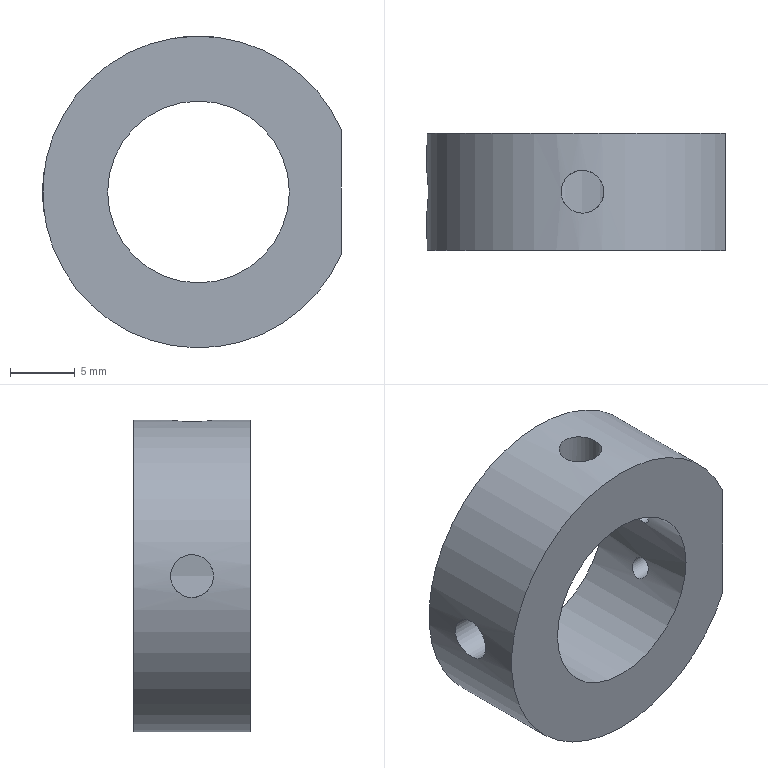Part | NX | 1 solid | 9 faces | box 23 x 9 x 24 mm | volume 2524 mm3 | cylinder 6 | plane 3 | commonest cylinder face diameters 1.6 x2 3.3 x2 14 x1 24 x1
STEP:
#1=CARTESIAN_POINT('',(11.,4.5,-4.796));
#2=VERTEX_POINT('',#1);
#3=CARTESIAN_POINT('',(11.,4.5,4.796));
#4=VERTEX_POINT('',#3);
#5=CARTESIAN_POINT('',(11.,4.5,10.));
#6=DIRECTION('',(0.,0.,1.));
#7=VECTOR('',#6,1000.);
#8=LINE('',#5,#7);
#9=EDGE_CURVE('',#2,#4,#8,.T.);
#10=ORIENTED_EDGE('',*,*,#9,.F.);
#11=CARTESIAN_POINT('',(0.,4.5,0.));
#12=DIRECTION('',(0.,1.,0.));
#13=DIRECTION('',(0.,0.,1.));
#14=AXIS2_PLACEMENT_3D('',#11,#12,#13);
#15=CIRCLE('',#14,12.);
#16=EDGE_CURVE('',#2,#4,#15,.T.);
#17=ORIENTED_EDGE('',*,*,#16,.T.);
#18=EDGE_LOOP('',(#10,#17));
#19=FACE_BOUND('',#18,.T.);
#20=CARTESIAN_POINT('',(0.,4.5,7.));
#21=VERTEX_POINT('',#20);
#22=CARTESIAN_POINT('',(0.,4.5,0.));
#23=DIRECTION('',(0.,1.,0.));
#24=DIRECTION('',(0.,0.,1.));
#25=AXIS2_PLACEMENT_3D('',#22,#23,#24);
#26=CIRCLE('',#25,7.);
#27=EDGE_CURVE('',#21,#21,#26,.T.);
#28=ORIENTED_EDGE('',*,*,#27,.F.);
#29=EDGE_LOOP('',(#28));
#30=FACE_BOUND('',#29,.T.);
#31=CARTESIAN_POINT('',(0.,4.5,0.));
#32=DIRECTION('',(0.,1.,0.));
#33=DIRECTION('',(0.,0.,1.));
#34=AXIS2_PLACEMENT_3D('',#31,#32,#33);
#35=PLANE('',#34);
#36=ADVANCED_FACE('',(#19,#30),#35,.T.);
#37=CARTESIAN_POINT('',(11.,-4.5,-4.796));
#38=VERTEX_POINT('',#37);
#39=CARTESIAN_POINT('',(11.,-4.5,4.796));
#40=VERTEX_POINT('',#39);
#41=CARTESIAN_POINT('',(0.,-4.5,0.));
#42=DIRECTION('',(0.,1.,0.));
#43=DIRECTION('',(0.,0.,1.));
#44=AXIS2_PLACEMENT_3D('',#41,#42,#43);
#45=CIRCLE('',#44,12.);
#46=EDGE_CURVE('',#38,#40,#45,.T.);
#47=ORIENTED_EDGE('',*,*,#46,.F.);
#48=CARTESIAN_POINT('',(11.,-4.5,0.));
#49=DIRECTION('',(0.,0.,1.));
#50=VECTOR('',#49,1000.);
#51=LINE('',#48,#50);
#52=EDGE_CURVE('',#38,#40,#51,.T.);
#53=ORIENTED_EDGE('',*,*,#52,.T.);
#54=EDGE_LOOP('',(#47,#53));
#55=FACE_BOUND('',#54,.T.);
#56=CARTESIAN_POINT('',(0.,-4.5,7.));
#57=VERTEX_POINT('',#56);
#58=CARTESIAN_POINT('',(0.,-4.5,0.));
#59=DIRECTION('',(0.,1.,0.));
#60=DIRECTION('',(0.,0.,1.));
#61=AXIS2_PLACEMENT_3D('',#58,#59,#60);
#62=CIRCLE('',#61,7.);
#63=EDGE_CURVE('',#57,#57,#62,.T.);
#64=ORIENTED_EDGE('',*,*,#63,.T.);
#65=EDGE_LOOP('',(#64));
#66=FACE_BOUND('',#65,.T.);
#67=CARTESIAN_POINT('',(0.,-4.5,0.));
#68=DIRECTION('',(0.,1.,0.));
#69=DIRECTION('',(0.,0.,1.));
#70=AXIS2_PLACEMENT_3D('',#67,#68,#69);
#71=PLANE('',#70);
#72=ADVANCED_FACE('',(#55,#66),#71,.F.);
#73=CARTESIAN_POINT('',(-12.,-1.65,0.));
#74=VERTEX_POINT('',#73);
#75=CARTESIAN_POINT('',(-11.943,-1.292,1.294));
#76=CARTESIAN_POINT('',(-12.028,-1.829,-0.000316));
#77=CARTESIAN_POINT('',(-11.943,-1.292,-1.293));
#78=CARTESIAN_POINT('',(-11.857,-0.001514,-1.828));
#79=CARTESIAN_POINT('',(-11.943,1.293,-1.294));
#80=CARTESIAN_POINT('',(-12.028,1.828,-0.0004038));
#81=CARTESIAN_POINT('',(-11.943,1.294,1.291));
#82=CARTESIAN_POINT('',(-11.857,0.00157,1.829));
#83=CARTESIAN_POINT('',(-11.943,-1.292,1.294));
#84=CARTESIAN_POINT('',(-12.028,-1.829,-0.000316));
#85=CARTESIAN_POINT('',(-11.943,-1.292,-1.293));
#86=B_SPLINE_CURVE_WITH_KNOTS('',3,(#75,#76,#77,#78,#79,#80,#81,#82,#83,#84,#85),.UNSPECIFIED.,.T.,.F.,(1,1,1,1,1,1,1,1,1,1,1,1,1,1,1),(-0.003873,-0.002582,-0.001291,0.,0.001291,0.002582,0.003873,0.005164,0.006455,0.007746,0.009037,0.01033,0.01162,0.01291,0.0142),.UNSPECIFIED.);
#87=EDGE_CURVE('',#74,#74,#86,.T.);
#88=ORIENTED_EDGE('',*,*,#87,.T.);
#89=EDGE_LOOP('',(#88));
#90=FACE_BOUND('',#89,.T.);
#91=CARTESIAN_POINT('',(0.,-1.65,12.));
#92=VERTEX_POINT('',#91);
#93=CARTESIAN_POINT('',(1.294,-1.292,11.943));
#94=CARTESIAN_POINT('',(-0.000316,-1.829,12.028));
#95=CARTESIAN_POINT('',(-1.293,-1.292,11.943));
#96=CARTESIAN_POINT('',(-1.828,-0.001514,11.857));
#97=CARTESIAN_POINT('',(-1.294,1.293,11.943));
#98=CARTESIAN_POINT('',(-0.0004038,1.828,12.028));
#99=CARTESIAN_POINT('',(1.291,1.294,11.943));
#100=CARTESIAN_POINT('',(1.829,0.00157,11.857));
#101=CARTESIAN_POINT('',(1.294,-1.292,11.943));
#102=CARTESIAN_POINT('',(-0.000316,-1.829,12.028));
#103=CARTESIAN_POINT('',(-1.293,-1.292,11.943));
#104=B_SPLINE_CURVE_WITH_KNOTS('',3,(#93,#94,#95,#96,#97,#98,#99,#100,#101,#102,#103),.UNSPECIFIED.,.T.,.F.,(1,1,1,1,1,1,1,1,1,1,1,1,1,1,1),(-0.003873,-0.002582,-0.001291,0.,0.001291,0.002582,0.003873,0.005164,0.006455,0.007746,0.009037,0.01033,0.01162,0.01291,0.0142),.UNSPECIFIED.);
#105=EDGE_CURVE('',#92,#92,#104,.T.);
#106=ORIENTED_EDGE('',*,*,#105,.T.);
#107=EDGE_LOOP('',(#106));
#108=FACE_BOUND('',#107,.T.);
#109=ORIENTED_EDGE('',*,*,#16,.F.);
#110=CARTESIAN_POINT('',(11.,4.5,-4.796));
#111=DIRECTION('',(0.,-1.,0.));
#112=VECTOR('',#111,1000.);
#113=LINE('',#110,#112);
#114=EDGE_CURVE('',#2,#38,#113,.T.);
#115=ORIENTED_EDGE('',*,*,#114,.T.);
#116=ORIENTED_EDGE('',*,*,#46,.T.);
#117=CARTESIAN_POINT('',(11.,4.5,4.796));
#118=DIRECTION('',(0.,-1.,0.));
#119=VECTOR('',#118,1000.);
#120=LINE('',#117,#119);
#121=EDGE_CURVE('',#40,#4,#120,.F.);
#122=ORIENTED_EDGE('',*,*,#121,.T.);
#123=EDGE_LOOP('',(#109,#115,#116,#122));
#124=FACE_BOUND('',#123,.T.);
#125=CARTESIAN_POINT('',(0.,4.5,0.));
#126=DIRECTION('',(0.,-1.,0.));
#127=DIRECTION('',(0.,0.,-1.));
#128=AXIS2_PLACEMENT_3D('',#125,#126,#127);
#129=CYLINDRICAL_SURFACE('',#128,12.);
#130=ADVANCED_FACE('',(#90,#108,#124),#129,.T.);
#131=CARTESIAN_POINT('',(-6.803,0.,-1.65));
#132=VERTEX_POINT('',#131);
#133=CARTESIAN_POINT('',(-6.903,-1.294,-1.292));
#134=CARTESIAN_POINT('',(-6.753,0.0002551,-1.829));
#135=CARTESIAN_POINT('',(-6.903,1.293,-1.292));
#136=CARTESIAN_POINT('',(-7.049,1.828,-0.001823));
#137=CARTESIAN_POINT('',(-6.903,1.293,1.293));
#138=CARTESIAN_POINT('',(-6.753,0.0007343,1.828));
#139=CARTESIAN_POINT('',(-6.903,-1.292,1.294));
#140=CARTESIAN_POINT('',(-7.049,-1.829,0.0008238));
#141=CARTESIAN_POINT('',(-6.903,-1.294,-1.292));
#142=CARTESIAN_POINT('',(-6.753,0.0002551,-1.829));
#143=CARTESIAN_POINT('',(-6.903,1.293,-1.292));
#144=B_SPLINE_CURVE_WITH_KNOTS('',3,(#133,#134,#135,#136,#137,#138,#139,#140,#141,#142,#143),.UNSPECIFIED.,.T.,.F.,(1,1,1,1,1,1,1,1,1,1,1,1,1,1,1),(-0.003882,-0.002588,-0.001294,0.,0.001294,0.002588,0.003882,0.005176,0.00647,0.007764,0.009058,0.01035,0.01165,0.01294,0.01423),.UNSPECIFIED.);
#145=EDGE_CURVE('',#132,#132,#144,.T.);
#146=ORIENTED_EDGE('',*,*,#145,.F.);
#147=EDGE_LOOP('',(#146));
#148=FACE_BOUND('',#147,.T.);
#149=CARTESIAN_POINT('',(-1.65,0.,6.803));
#150=VERTEX_POINT('',#149);
#151=CARTESIAN_POINT('',(-1.292,-1.294,6.903));
#152=CARTESIAN_POINT('',(-1.829,0.0002551,6.753));
#153=CARTESIAN_POINT('',(-1.292,1.293,6.903));
#154=CARTESIAN_POINT('',(-0.001823,1.828,7.049));
#155=CARTESIAN_POINT('',(1.293,1.293,6.903));
#156=CARTESIAN_POINT('',(1.828,0.0007343,6.753));
#157=CARTESIAN_POINT('',(1.294,-1.292,6.903));
#158=CARTESIAN_POINT('',(0.0008238,-1.829,7.049));
#159=CARTESIAN_POINT('',(-1.292,-1.294,6.903));
#160=CARTESIAN_POINT('',(-1.829,0.0002551,6.753));
#161=CARTESIAN_POINT('',(-1.292,1.293,6.903));
#162=B_SPLINE_CURVE_WITH_KNOTS('',3,(#151,#152,#153,#154,#155,#156,#157,#158,#159,#160,#161),.UNSPECIFIED.,.T.,.F.,(1,1,1,1,1,1,1,1,1,1,1,1,1,1,1),(-0.003882,-0.002588,-0.001294,0.,0.001294,0.002588,0.003882,0.005176,0.00647,0.007764,0.009058,0.01035,0.01165,0.01294,0.01423),.UNSPECIFIED.);
#163=EDGE_CURVE('',#150,#150,#162,.T.);
#164=ORIENTED_EDGE('',*,*,#163,.F.);
#165=EDGE_LOOP('',(#164));
#166=FACE_BOUND('',#165,.T.);
#167=CARTESIAN_POINT('',(6.79,0.,1.7));
#168=VERTEX_POINT('',#167);
#169=CARTESIAN_POINT('',(6.746,0.6498,1.892));
#170=CARTESIAN_POINT('',(6.813,-0.0002908,1.604));
#171=CARTESIAN_POINT('',(6.746,-0.6486,1.891));
#172=CARTESIAN_POINT('',(6.544,-0.8781,2.519));
#173=CARTESIAN_POINT('',(6.278,-0.6383,3.11));
#174=CARTESIAN_POINT('',(6.121,-0.002448,3.394));
#175=CARTESIAN_POINT('',(6.277,0.6376,3.112));
#176=CARTESIAN_POINT('',(6.544,0.878,2.519));
#177=CARTESIAN_POINT('',(6.746,0.6498,1.892));
#178=CARTESIAN_POINT('',(6.813,-0.0002908,1.604));
#179=CARTESIAN_POINT('',(6.746,-0.6486,1.891));
#180=B_SPLINE_CURVE_WITH_KNOTS('',3,(#169,#170,#171,#172,#173,#174,#175,#176,#177,#178,#179),.UNSPECIFIED.,.T.,.F.,(1,1,1,1,1,1,1,1,1,1,1,1,1,1,1),(-0.001946,-0.001297,-0.0006485,0.,0.0006485,0.001297,0.001946,0.002594,0.003243,0.003891,0.00454,0.005188,0.005837,0.006485,0.007134),.UNSPECIFIED.);
#181=EDGE_CURVE('',#168,#168,#180,.T.);
#182=ORIENTED_EDGE('',*,*,#181,.F.);
#183=EDGE_LOOP('',(#182));
#184=FACE_BOUND('',#183,.T.);
#185=CARTESIAN_POINT('',(6.173,0.,-3.3));
#186=VERTEX_POINT('',#185);
#187=CARTESIAN_POINT('',(6.278,0.6381,-3.111));
#188=CARTESIAN_POINT('',(6.121,0.0001146,-3.395));
#189=CARTESIAN_POINT('',(6.278,-0.6385,-3.111));
#190=CARTESIAN_POINT('',(6.544,-0.8779,-2.519));
#191=CARTESIAN_POINT('',(6.746,-0.6493,-1.892));
#192=CARTESIAN_POINT('',(6.813,-0.000522,-1.605));
#193=CARTESIAN_POINT('',(6.746,0.6482,-1.89));
#194=CARTESIAN_POINT('',(6.544,0.8783,-2.52));
#195=CARTESIAN_POINT('',(6.278,0.6381,-3.111));
#196=CARTESIAN_POINT('',(6.121,0.0001146,-3.395));
#197=CARTESIAN_POINT('',(6.278,-0.6385,-3.111));
#198=B_SPLINE_CURVE_WITH_KNOTS('',3,(#187,#188,#189,#190,#191,#192,#193,#194,#195,#196,#197),.UNSPECIFIED.,.T.,.F.,(1,1,1,1,1,1,1,1,1,1,1,1,1,1,1),(-0.001946,-0.001297,-0.0006486,0.,0.0006486,0.001297,0.001946,0.002594,0.003243,0.003892,0.00454,0.005189,0.005838,0.006486,0.007135),.UNSPECIFIED.);
#199=EDGE_CURVE('',#186,#186,#198,.T.);
#200=ORIENTED_EDGE('',*,*,#199,.F.);
#201=EDGE_LOOP('',(#200));
#202=FACE_BOUND('',#201,.T.);
#203=ORIENTED_EDGE('',*,*,#27,.T.);
#204=EDGE_LOOP('',(#203));
#205=FACE_BOUND('',#204,.T.);
#206=ORIENTED_EDGE('',*,*,#63,.F.);
#207=EDGE_LOOP('',(#206));
#208=FACE_BOUND('',#207,.T.);
#209=CARTESIAN_POINT('',(0.,4.5,0.));
#210=DIRECTION('',(0.,-1.,0.));
#211=DIRECTION('',(0.,0.,-1.));
#212=AXIS2_PLACEMENT_3D('',#209,#210,#211);
#213=CYLINDRICAL_SURFACE('',#212,7.);
#214=ADVANCED_FACE('',(#148,#166,#184,#202,#205,#208),#213,.F.);
#215=CARTESIAN_POINT('',(11.,0.,1.7));
#216=VERTEX_POINT('',#215);
#217=CARTESIAN_POINT('',(11.,0.,2.5));
#218=DIRECTION('',(1.,0.,0.));
#219=DIRECTION('',(0.,0.,-1.));
#220=AXIS2_PLACEMENT_3D('',#217,#218,#219);
#221=CIRCLE('',#220,0.8);
#222=EDGE_CURVE('',#216,#216,#221,.T.);
#223=ORIENTED_EDGE('',*,*,#222,.F.);
#224=EDGE_LOOP('',(#223));
#225=FACE_BOUND('',#224,.T.);
#226=CARTESIAN_POINT('',(11.,0.,-3.3));
#227=VERTEX_POINT('',#226);
#228=CARTESIAN_POINT('',(11.,0.,-2.5));
#229=DIRECTION('',(1.,0.,0.));
#230=DIRECTION('',(0.,0.,-1.));
#231=AXIS2_PLACEMENT_3D('',#228,#229,#230);
#232=CIRCLE('',#231,0.8);
#233=EDGE_CURVE('',#227,#227,#232,.T.);
#234=ORIENTED_EDGE('',*,*,#233,.F.);
#235=EDGE_LOOP('',(#234));
#236=FACE_BOUND('',#235,.T.);
#237=ORIENTED_EDGE('',*,*,#9,.T.);
#238=ORIENTED_EDGE('',*,*,#121,.F.);
#239=ORIENTED_EDGE('',*,*,#52,.F.);
#240=ORIENTED_EDGE('',*,*,#114,.F.);
#241=EDGE_LOOP('',(#237,#238,#239,#240));
#242=FACE_BOUND('',#241,.T.);
#243=CARTESIAN_POINT('',(11.,-20.5,10.));
#244=DIRECTION('',(-1.,0.,0.));
#245=DIRECTION('',(0.,0.,1.));
#246=AXIS2_PLACEMENT_3D('',#243,#244,#245);
#247=PLANE('',#246);
#248=ADVANCED_FACE('',(#225,#236,#242),#247,.F.);
#249=ORIENTED_EDGE('',*,*,#199,.T.);
#250=EDGE_LOOP('',(#249));
#251=FACE_BOUND('',#250,.T.);
#252=ORIENTED_EDGE('',*,*,#233,.T.);
#253=EDGE_LOOP('',(#252));
#254=FACE_BOUND('',#253,.T.);
#255=CARTESIAN_POINT('',(11.,0.,-2.5));
#256=DIRECTION('',(1.,0.,0.));
#257=DIRECTION('',(0.,0.,-1.));
#258=AXIS2_PLACEMENT_3D('',#255,#256,#257);
#259=CYLINDRICAL_SURFACE('',#258,0.8);
#260=ADVANCED_FACE('',(#251,#254),#259,.F.);
#261=ORIENTED_EDGE('',*,*,#181,.T.);
#262=EDGE_LOOP('',(#261));
#263=FACE_BOUND('',#262,.T.);
#264=ORIENTED_EDGE('',*,*,#222,.T.);
#265=EDGE_LOOP('',(#264));
#266=FACE_BOUND('',#265,.T.);
#267=CARTESIAN_POINT('',(11.,0.,2.5));
#268=DIRECTION('',(1.,0.,0.));
#269=DIRECTION('',(0.,0.,-1.));
#270=AXIS2_PLACEMENT_3D('',#267,#268,#269);
#271=CYLINDRICAL_SURFACE('',#270,0.8);
#272=ADVANCED_FACE('',(#263,#266),#271,.F.);
#273=ORIENTED_EDGE('',*,*,#163,.T.);
#274=EDGE_LOOP('',(#273));
#275=FACE_BOUND('',#274,.T.);
#276=ORIENTED_EDGE('',*,*,#105,.F.);
#277=EDGE_LOOP('',(#276));
#278=FACE_BOUND('',#277,.T.);
#279=CARTESIAN_POINT('',(0.,0.,0.));
#280=DIRECTION('',(0.,0.,-1.));
#281=DIRECTION('',(-1.,0.,0.));
#282=AXIS2_PLACEMENT_3D('',#279,#280,#281);
#283=CYLINDRICAL_SURFACE('',#282,1.65);
#284=ADVANCED_FACE('',(#275,#278),#283,.F.);
#285=ORIENTED_EDGE('',*,*,#145,.T.);
#286=EDGE_LOOP('',(#285));
#287=FACE_BOUND('',#286,.T.);
#288=ORIENTED_EDGE('',*,*,#87,.F.);
#289=EDGE_LOOP('',(#288));
#290=FACE_BOUND('',#289,.T.);
#291=CARTESIAN_POINT('',(0.,0.,0.));
#292=DIRECTION('',(1.,0.,0.));
#293=DIRECTION('',(0.,0.,-1.));
#294=AXIS2_PLACEMENT_3D('',#291,#292,#293);
#295=CYLINDRICAL_SURFACE('',#294,1.65);
#296=ADVANCED_FACE('',(#287,#290),#295,.F.);
#297=CLOSED_SHELL('',(#36,#72,#130,#214,#248,#260,#272,#284,#296));
#298=MANIFOLD_SOLID_BREP('',#297);
#299=(LENGTH_UNIT()NAMED_UNIT(*)SI_UNIT(.MILLI.,.METRE.));
#300=UNCERTAINTY_MEASURE_WITH_UNIT(LENGTH_MEASURE(0.0508),#299,'','');
#301=(NAMED_UNIT(*)PLANE_ANGLE_UNIT()SI_UNIT($,.RADIAN.));
#302=(NAMED_UNIT(*)SI_UNIT($,.STERADIAN.)SOLID_ANGLE_UNIT());
#303=(GEOMETRIC_REPRESENTATION_CONTEXT(3)GLOBAL_UNCERTAINTY_ASSIGNED_CONTEXT((#300))GLOBAL_UNIT_ASSIGNED_CONTEXT((#299,#301,#302))REPRESENTATION_CONTEXT('',''));
#304=ADVANCED_BREP_SHAPE_REPRESENTATION('',(#298),#303);